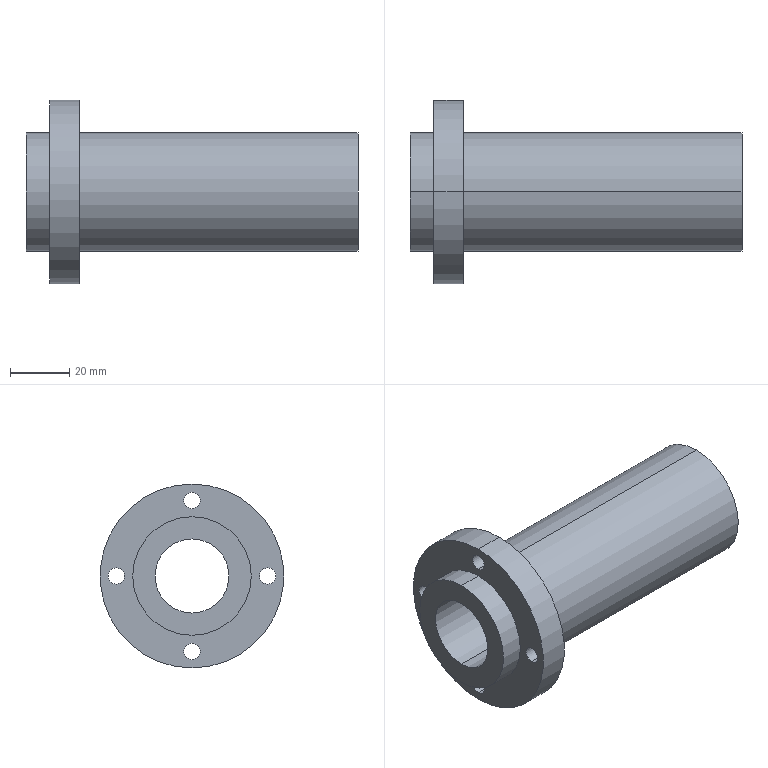Part | STEP file | Linear bearing LMFP25LUU | 1 solid | 32 faces | box 112 x 62 x 62 mm | volume 101190 mm3 | cylinder 24 | plane 8 | commonest cylinder face diameters 5.5 x8 10 x8 40 x4 25 x2 62 x2